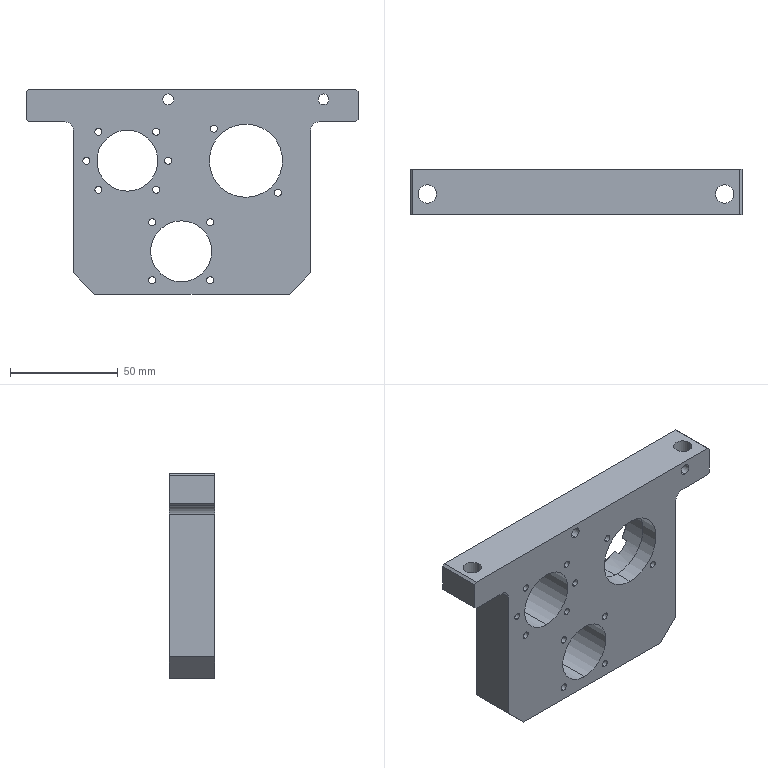Part | STEP file | Right Moving Support Plate | 1 solid | 67 faces | box 154 x 21 x 95 mm | volume 178723 mm3 | cylinder 45 | plane 19 | cone 3 | commonest cylinder face diameters 3.3 x24 5 x4 8.5 x4 28.3 x4 9 x3 8 x2